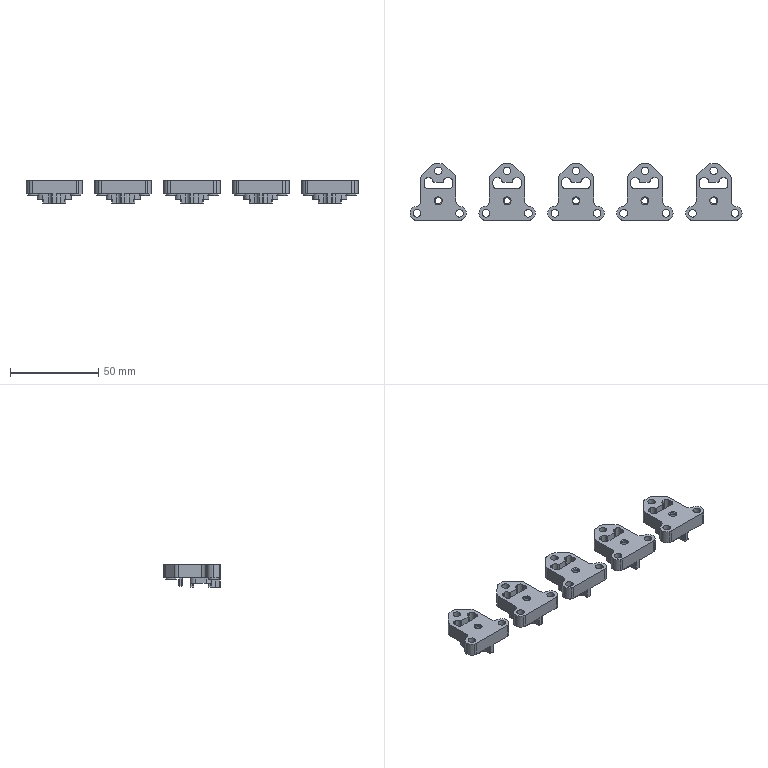CAM job | NX | 3-axis milling | part box 188 x 32 x 13 mm | stock box 192 x 36 x 14 mm
Tools:
number,name,description,diameter,corner_radius,flute_length,length,flutes
19,D80,Milling Tool-5 Parameters,80.0,0.0,50.0,75.0,2
12,D6,Milling Tool-5 Parameters,6.0,0.0,50.0,75.0,2
16,D3,Milling Tool-5 Parameters,3.0,0.0,50.0,75.0,2
11,D4,Milling Tool-5 Parameters,4.0,0.0,50.0,75.0,2
2,D2,Milling Tool-5 Parameters,2.0,0.0,50.0,75.0,2
17,D1,Milling Tool-5 Parameters,1.0,0.0,50.0,75.0,2
18,D2R0.5,Milling Tool-5 Parameters,2.0,0.5,50.0,75.0,2
9,D0.5,Milling Tool-5 Parameters,0.5,0.0,50.0,75.0,2
Operations:
program,operation,operation_type,tool,method,geometry_group,spindle_rpm,surface_speed,feed_per_tooth,feed_cut,feed_plunge,cut_length_mm,path_length_mm,cut_time_min,machine_time_min
1AB胶,FLOOR_WALL,VolumeBased25DMillingOperation,D80,METHOD,A,6500.0,1633.0,0.1154,1500.0,100.0,284.0,338.0,0.1893,0.1947
1AB胶,ZLEVEL_PROFILE,ZLevelMilling,D6,METHOD,A,9500.0,298.0,0.1579,3000.0,1000.0,14441.98,15211.641,4.947,5.024
1AB胶,CAVITY_MILL,CavityMilling,D4,METHOD,A,9500.0,119.0,0.1316,2500.0,1000.0,43967.957,48380.703,22.652,23.094
1AB胶,CAVITY_MILL_COPY,CavityMilling,D3,METHOD,A,9500.0,89.0,0.0947,1800.0,1000.0,8021.355,12840.271,5.211,5.693
1AB胶,HOLE_MILLING,CylinderMilling,D3,METHOD,A,9500.0,59.0,0.0526,1000.0,100.0,3810.901,5287.78,3.811,3.959
1AB胶,FLOOR_WALL_1_COPY,VolumeBased25DMillingOperation,D3,METHOD,A,9500.0,89.0,0.0711,1350.0,100.0,388.0,1010.0,0.2874,0.3496
1AB胶,ZLEVEL_PROFILE_COPY,ZLevelMilling,D3,METHOD,A,9500.0,89.0,0.0632,1200.0,1000.0,532.801,1833.916,0.4498,0.5799
1AB胶,FLOOR_WALL_1,VolumeBased25DMillingOperation,D3,METHOD,A,9500.0,89.0,0.0711,1350.0,100.0,4463.5,10776.663,3.306,3.938
1AB胶,CAVITY_MILL_COPY_COPY,CavityMilling,D2,METHOD,A,9500.0,59.0,0.0579,1100.0,1000.0,4035.238,8717.154,3.787,4.255
1AB胶,CAVITY_MILL_COPY_COPY_COPY,CavityMilling,D1,METHOD,A,9500.0,29.0,0.0421,800.0,1000.0,2128.142,5011.106,2.551,2.839
1AB胶,CAVITY_MILL_COPY_COPY_COPY_COPY,CavityMilling,D0.5,METHOD,A,9500.0,14.0,0.0368,700.0,1000.0,2120.385,20755.673,2.871,4.735
1AB胶,FIXED_CONTOUR,SurfaceContour,D2R0.5,METHOD,A,9500.0,59.0,0.1316,2500.0,100.0,5038.706,9795.318,2.015,2.491
1AB胶,刀补,ZLevelMilling,D0.5,METHOD,A,9500.0,29.0,0.0526,1000.0,1000.0,358.436,1752.768,0.3584,0.4979
1AB胶,ZLEVEL_PROFILE_COPY_1,ZLevelMilling,D6,METHOD,A,9500.0,298.0,0.0632,1200.0,1000.0,3383.782,4364.693,2.846,2.944